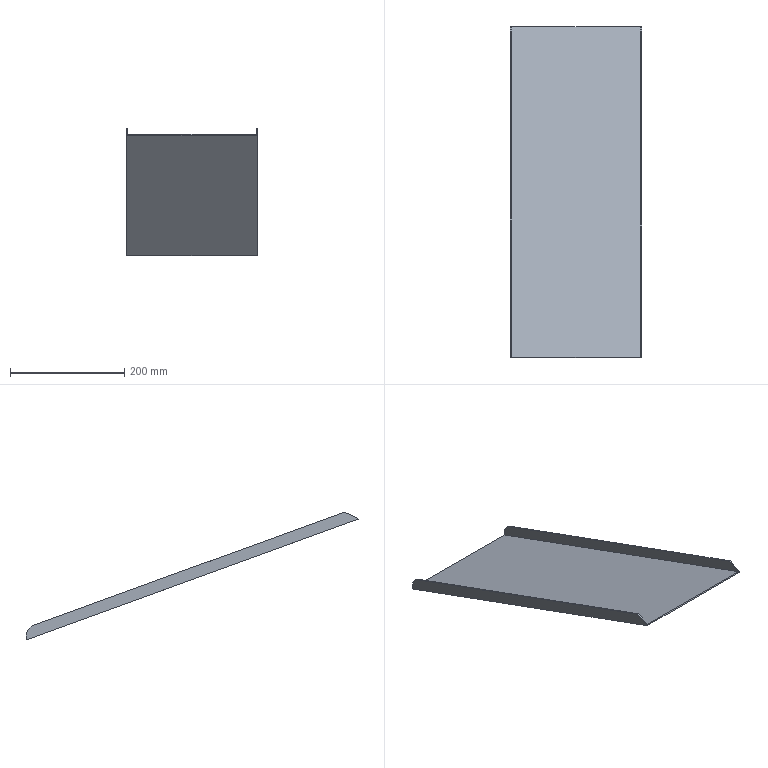Part | NX | features solid 2 | 1 solid | 15 faces | box 229.044 x 580.567 x 223.508 mm | volume 325645 mm3 | plane 13 | cylinder 2 | commonest cylinder face diameters 40 x2
STEP:
#1=CARTESIAN_POINT('',(-7.044,820.,-511.765));
#2=VERTEX_POINT('',#1);
#3=CARTESIAN_POINT('',(218.,820.,-511.765));
#4=VERTEX_POINT('',#3);
#5=CARTESIAN_POINT('',(-4.044,820.,-511.765));
#6=DIRECTION('',(-1.,0.,0.));
#7=VECTOR('',#6,1000.);
#8=LINE('',#5,#7);
#9=EDGE_CURVE('',#2,#4,#8,.F.);
#10=ORIENTED_EDGE('',*,*,#9,.F.);
#11=CARTESIAN_POINT('',(-7.044,820.,-509.637));
#12=VERTEX_POINT('',#11);
#13=CARTESIAN_POINT('',(-7.044,820.,-700.));
#14=DIRECTION('',(0.,0.,-1.));
#15=VECTOR('',#14,1000.);
#16=LINE('',#13,#15);
#17=EDGE_CURVE('',#2,#12,#16,.F.);
#18=ORIENTED_EDGE('',*,*,#17,.T.);
#19=CARTESIAN_POINT('',(218.,820.,-509.637));
#20=VERTEX_POINT('',#19);
#21=CARTESIAN_POINT('',(1065.,820.,-509.637));
#22=DIRECTION('',(1.,0.,0.));
#23=VECTOR('',#22,1000.);
#24=LINE('',#21,#23);
#25=EDGE_CURVE('',#20,#12,#24,.F.);
#26=ORIENTED_EDGE('',*,*,#25,.F.);
#27=CARTESIAN_POINT('',(218.,820.,-700.));
#28=DIRECTION('',(0.,0.,-1.));
#29=VECTOR('',#28,1000.);
#30=LINE('',#27,#29);
#31=EDGE_CURVE('',#4,#20,#30,.F.);
#32=ORIENTED_EDGE('',*,*,#31,.F.);
#33=EDGE_LOOP('',(#10,#18,#26,#32));
#34=FACE_BOUND('',#33,.T.);
#35=CARTESIAN_POINT('',(1065.,820.,-700.));
#36=DIRECTION('',(0.,-1.,0.));
#37=DIRECTION('',(-1.,0.,0.));
#38=AXIS2_PLACEMENT_3D('',#35,#36,#37);
#39=PLANE('',#38);
#40=ADVANCED_FACE('',(#34),#39,.F.);
#41=CARTESIAN_POINT('',(218.,241.366,-299.031));
#42=VERTEX_POINT('',#41);
#43=CARTESIAN_POINT('',(-7.044,241.366,-299.031));
#44=VERTEX_POINT('',#43);
#45=CARTESIAN_POINT('',(-4.044,241.366,-299.031));
#46=DIRECTION('',(-1.,0.,0.));
#47=VECTOR('',#46,1000.);
#48=LINE('',#45,#47);
#49=EDGE_CURVE('',#42,#44,#48,.T.);
#50=ORIENTED_EDGE('',*,*,#49,.T.);
#51=CARTESIAN_POINT('',(-7.044,240.682,-300.911));
#52=VERTEX_POINT('',#51);
#53=CARTESIAN_POINT('',(-7.044,240.682,-300.911));
#54=DIRECTION('',(0.,-0.342,-0.9397));
#55=VECTOR('',#54,1000.);
#56=LINE('',#53,#55);
#57=EDGE_CURVE('',#44,#52,#56,.T.);
#58=ORIENTED_EDGE('',*,*,#57,.T.);
#59=CARTESIAN_POINT('',(220.,240.682,-300.911));
#60=VERTEX_POINT('',#59);
#61=CARTESIAN_POINT('',(-4.044,240.682,-300.911));
#62=DIRECTION('',(-1.,0.,0.));
#63=VECTOR('',#62,1000.);
#64=LINE('',#61,#63);
#65=EDGE_CURVE('',#60,#52,#64,.T.);
#66=ORIENTED_EDGE('',*,*,#65,.F.);
#67=CARTESIAN_POINT('',(220.,241.366,-299.031));
#68=VERTEX_POINT('',#67);
#69=CARTESIAN_POINT('',(220.,241.366,-299.031));
#70=DIRECTION('',(0.,-0.342,-0.9397));
#71=VECTOR('',#70,1000.);
#72=LINE('',#69,#71);
#73=EDGE_CURVE('',#68,#60,#72,.T.);
#74=ORIENTED_EDGE('',*,*,#73,.F.);
#75=CARTESIAN_POINT('',(-4.044,241.366,-299.031));
#76=DIRECTION('',(-1.,0.,0.));
#77=VECTOR('',#76,1000.);
#78=LINE('',#75,#77);
#79=EDGE_CURVE('',#68,#42,#78,.T.);
#80=ORIENTED_EDGE('',*,*,#79,.T.);
#81=EDGE_LOOP('',(#50,#58,#66,#74,#80));
#82=FACE_BOUND('',#81,.T.);
#83=CARTESIAN_POINT('',(220.,240.682,-300.911));
#84=DIRECTION('',(0.,-0.9397,0.342));
#85=DIRECTION('',(0.,0.342,0.9397));
#86=AXIS2_PLACEMENT_3D('',#83,#84,#85);
#87=PLANE('',#86);
#88=ADVANCED_FACE('',(#82),#87,.T.);
#89=CARTESIAN_POINT('',(-7.044,1206.032,-650.141));
#90=DIRECTION('',(0.,0.9397,-0.342));
#91=VECTOR('',#90,1000.);
#92=LINE('',#89,#91);
#93=EDGE_CURVE('',#44,#12,#92,.T.);
#94=ORIENTED_EDGE('',*,*,#93,.F.);
#95=ORIENTED_EDGE('',*,*,#49,.F.);
#96=CARTESIAN_POINT('',(218.,1206.032,-650.141));
#97=DIRECTION('',(0.,0.9397,-0.342));
#98=VECTOR('',#97,1000.);
#99=LINE('',#96,#98);
#100=EDGE_CURVE('',#42,#20,#99,.T.);
#101=ORIENTED_EDGE('',*,*,#100,.T.);
#102=ORIENTED_EDGE('',*,*,#25,.T.);
#103=EDGE_LOOP('',(#94,#95,#101,#102));
#104=FACE_BOUND('',#103,.T.);
#105=CARTESIAN_POINT('',(-4.044,1206.032,-650.141));
#106=DIRECTION('',(0.,-0.342,-0.9397));
#107=DIRECTION('',(-1.,0.,0.));
#108=AXIS2_PLACEMENT_3D('',#105,#106,#107);
#109=PLANE('',#108);
#110=ADVANCED_FACE('',(#104),#109,.F.);
#111=CARTESIAN_POINT('',(220.,820.,-511.765));
#112=VERTEX_POINT('',#111);
#113=CARTESIAN_POINT('',(220.,1205.348,-652.02));
#114=DIRECTION('',(0.,-0.9397,0.342));
#115=VECTOR('',#114,1000.);
#116=LINE('',#113,#115);
#117=EDGE_CURVE('',#112,#60,#116,.T.);
#118=ORIENTED_EDGE('',*,*,#117,.F.);
#119=CARTESIAN_POINT('',(220.,808.047,-486.131));
#120=VERTEX_POINT('',#119);
#121=CARTESIAN_POINT('',(220.,801.206,-504.925));
#122=DIRECTION('',(-1.,0.,0.));
#123=DIRECTION('',(0.,0.,1.));
#124=AXIS2_PLACEMENT_3D('',#121,#122,#123);
#125=CIRCLE('',#124,20.);
#126=EDGE_CURVE('',#112,#120,#125,.F.);
#127=ORIENTED_EDGE('',*,*,#126,.T.);
#128=CARTESIAN_POINT('',(220.,264.437,-288.273));
#129=VERTEX_POINT('',#128);
#130=CARTESIAN_POINT('',(220.,826.84,-492.971));
#131=DIRECTION('',(0.,-0.9397,0.342));
#132=VECTOR('',#131,1000.);
#133=LINE('',#130,#132);
#134=EDGE_CURVE('',#120,#129,#133,.T.);
#135=ORIENTED_EDGE('',*,*,#134,.T.);
#136=CARTESIAN_POINT('',(220.,241.366,-299.031));
#137=DIRECTION('',(0.,-0.9063,-0.4226));
#138=VECTOR('',#137,1000.);
#139=LINE('',#136,#138);
#140=EDGE_CURVE('',#129,#68,#139,.T.);
#141=ORIENTED_EDGE('',*,*,#140,.T.);
#142=ORIENTED_EDGE('',*,*,#73,.T.);
#143=EDGE_LOOP('',(#118,#127,#135,#141,#142));
#144=FACE_BOUND('',#143,.T.);
#145=CARTESIAN_POINT('',(220.,1206.032,-650.141));
#146=DIRECTION('',(1.,0.,0.));
#147=DIRECTION('',(0.,0.,-1.));
#148=AXIS2_PLACEMENT_3D('',#145,#146,#147);
#149=PLANE('',#148);
#150=ADVANCED_FACE('',(#144),#149,.T.);
#151=CARTESIAN_POINT('',(-9.044,808.047,-486.131));
#152=VERTEX_POINT('',#151);
#153=CARTESIAN_POINT('',(-9.044,820.,-511.765));
#154=VERTEX_POINT('',#153);
#155=CARTESIAN_POINT('',(-9.044,801.206,-504.925));
#156=DIRECTION('',(-1.,0.,0.));
#157=DIRECTION('',(0.,0.,1.));
#158=AXIS2_PLACEMENT_3D('',#155,#156,#157);
#159=CIRCLE('',#158,20.);
#160=EDGE_CURVE('',#152,#154,#159,.T.);
#161=ORIENTED_EDGE('',*,*,#160,.T.);
#162=CARTESIAN_POINT('',(-9.044,240.639,-300.895));
#163=VERTEX_POINT('',#162);
#164=CARTESIAN_POINT('',(-9.044,1205.348,-652.02));
#165=DIRECTION('',(0.,-0.9397,0.342));
#166=VECTOR('',#165,1000.);
#167=LINE('',#164,#166);
#168=EDGE_CURVE('',#154,#163,#167,.T.);
#169=ORIENTED_EDGE('',*,*,#168,.T.);
#170=CARTESIAN_POINT('',(-9.044,241.323,-299.015));
#171=VERTEX_POINT('',#170);
#172=CARTESIAN_POINT('',(-9.044,240.639,-300.895));
#173=DIRECTION('',(0.,0.342,0.9397));
#174=VECTOR('',#173,1000.);
#175=LINE('',#172,#174);
#176=EDGE_CURVE('',#163,#171,#175,.T.);
#177=ORIENTED_EDGE('',*,*,#176,.T.);
#178=CARTESIAN_POINT('',(-9.044,264.394,-288.257));
#179=VERTEX_POINT('',#178);
#180=CARTESIAN_POINT('',(-9.044,635.157,-115.368));
#181=DIRECTION('',(0.,0.9063,0.4226));
#182=VECTOR('',#181,1000.);
#183=LINE('',#180,#182);
#184=EDGE_CURVE('',#171,#179,#183,.T.);
#185=ORIENTED_EDGE('',*,*,#184,.T.);
#186=CARTESIAN_POINT('',(-9.044,826.84,-492.971));
#187=DIRECTION('',(0.,-0.9397,0.342));
#188=VECTOR('',#187,1000.);
#189=LINE('',#186,#188);
#190=EDGE_CURVE('',#152,#179,#189,.T.);
#191=ORIENTED_EDGE('',*,*,#190,.F.);
#192=EDGE_LOOP('',(#161,#169,#177,#185,#191));
#193=FACE_BOUND('',#192,.T.);
#194=CARTESIAN_POINT('',(-9.044,1206.032,-650.141));
#195=DIRECTION('',(1.,0.,0.));
#196=DIRECTION('',(0.,0.,-1.));
#197=AXIS2_PLACEMENT_3D('',#194,#195,#196);
#198=PLANE('',#197);
#199=ADVANCED_FACE('',(#193),#198,.F.);
#200=CARTESIAN_POINT('',(-4.044,820.,-511.765));
#201=DIRECTION('',(-1.,0.,0.));
#202=VECTOR('',#201,1000.);
#203=LINE('',#200,#202);
#204=EDGE_CURVE('',#154,#2,#203,.F.);
#205=ORIENTED_EDGE('',*,*,#204,.T.);
#206=ORIENTED_EDGE('',*,*,#9,.T.);
#207=CARTESIAN_POINT('',(220.,820.,-511.765));
#208=DIRECTION('',(1.,0.,0.));
#209=VECTOR('',#208,1000.);
#210=LINE('',#207,#209);
#211=EDGE_CURVE('',#112,#4,#210,.F.);
#212=ORIENTED_EDGE('',*,*,#211,.F.);
#213=ORIENTED_EDGE('',*,*,#117,.T.);
#214=ORIENTED_EDGE('',*,*,#65,.T.);
#215=CARTESIAN_POINT('',(-7.044,240.639,-300.895));
#216=VERTEX_POINT('',#215);
#217=CARTESIAN_POINT('',(-7.044,820.,-511.765));
#218=DIRECTION('',(0.,-0.9397,0.342));
#219=VECTOR('',#218,1000.);
#220=LINE('',#217,#219);
#221=EDGE_CURVE('',#52,#216,#220,.T.);
#222=ORIENTED_EDGE('',*,*,#221,.T.);
#223=CARTESIAN_POINT('',(-9.044,240.639,-300.895));
#224=DIRECTION('',(1.,0.,0.));
#225=VECTOR('',#224,1000.);
#226=LINE('',#223,#225);
#227=EDGE_CURVE('',#163,#216,#226,.T.);
#228=ORIENTED_EDGE('',*,*,#227,.F.);
#229=ORIENTED_EDGE('',*,*,#168,.F.);
#230=EDGE_LOOP('',(#205,#206,#212,#213,#214,#222,#228,#229));
#231=FACE_BOUND('',#230,.T.);
#232=CARTESIAN_POINT('',(-4.044,1205.348,-652.02));
#233=DIRECTION('',(0.,-0.342,-0.9397));
#234=DIRECTION('',(-1.,0.,0.));
#235=AXIS2_PLACEMENT_3D('',#232,#233,#234);
#236=PLANE('',#235);
#237=ADVANCED_FACE('',(#231),#236,.T.);
#238=CARTESIAN_POINT('',(218.,808.047,-486.131));
#239=VERTEX_POINT('',#238);
#240=CARTESIAN_POINT('',(218.,264.437,-288.273));
#241=VERTEX_POINT('',#240);
#242=CARTESIAN_POINT('',(218.,826.84,-492.971));
#243=DIRECTION('',(0.,-0.9397,0.342));
#244=VECTOR('',#243,1000.);
#245=LINE('',#242,#244);
#246=EDGE_CURVE('',#239,#241,#245,.T.);
#247=ORIENTED_EDGE('',*,*,#246,.T.);
#248=CARTESIAN_POINT('',(220.,264.437,-288.273));
#249=DIRECTION('',(1.,0.,0.));
#250=VECTOR('',#249,1000.);
#251=LINE('',#248,#250);
#252=EDGE_CURVE('',#241,#129,#251,.T.);
#253=ORIENTED_EDGE('',*,*,#252,.T.);
#254=ORIENTED_EDGE('',*,*,#134,.F.);
#255=CARTESIAN_POINT('',(220.,808.047,-486.131));
#256=DIRECTION('',(-1.,0.,0.));
#257=VECTOR('',#256,1000.);
#258=LINE('',#255,#257);
#259=EDGE_CURVE('',#120,#239,#258,.T.);
#260=ORIENTED_EDGE('',*,*,#259,.T.);
#261=EDGE_LOOP('',(#247,#253,#254,#260));
#262=FACE_BOUND('',#261,.T.);
#263=CARTESIAN_POINT('',(220.,826.84,-492.971));
#264=DIRECTION('',(0.,-0.342,-0.9397));
#265=DIRECTION('',(0.,-0.9397,0.342));
#266=AXIS2_PLACEMENT_3D('',#263,#264,#265);
#267=PLANE('',#266);
#268=ADVANCED_FACE('',(#262),#267,.F.);
#269=CARTESIAN_POINT('',(218.,801.206,-504.925));
#270=DIRECTION('',(-1.,0.,0.));
#271=DIRECTION('',(0.,0.,1.));
#272=AXIS2_PLACEMENT_3D('',#269,#270,#271);
#273=CIRCLE('',#272,20.);
#274=EDGE_CURVE('',#239,#4,#273,.T.);
#275=ORIENTED_EDGE('',*,*,#274,.T.);
#276=ORIENTED_EDGE('',*,*,#31,.T.);
#277=ORIENTED_EDGE('',*,*,#100,.F.);
#278=CARTESIAN_POINT('',(218.,635.171,-115.397));
#279=DIRECTION('',(0.,0.9063,0.4226));
#280=VECTOR('',#279,1000.);
#281=LINE('',#278,#280);
#282=EDGE_CURVE('',#42,#241,#281,.T.);
#283=ORIENTED_EDGE('',*,*,#282,.T.);
#284=ORIENTED_EDGE('',*,*,#246,.F.);
#285=EDGE_LOOP('',(#275,#276,#277,#283,#284));
#286=FACE_BOUND('',#285,.T.);
#287=CARTESIAN_POINT('',(218.,820.,-511.765));
#288=DIRECTION('',(-1.,0.,0.));
#289=DIRECTION('',(0.,0.,1.));
#290=AXIS2_PLACEMENT_3D('',#287,#288,#289);
#291=PLANE('',#290);
#292=ADVANCED_FACE('',(#286),#291,.T.);
#293=ORIENTED_EDGE('',*,*,#126,.F.);
#294=ORIENTED_EDGE('',*,*,#211,.T.);
#295=ORIENTED_EDGE('',*,*,#274,.F.);
#296=ORIENTED_EDGE('',*,*,#259,.F.);
#297=EDGE_LOOP('',(#293,#294,#295,#296));
#298=FACE_BOUND('',#297,.T.);
#299=CARTESIAN_POINT('',(220.,801.206,-504.925));
#300=DIRECTION('',(-1.,0.,0.));
#301=DIRECTION('',(0.,0.,1.));
#302=AXIS2_PLACEMENT_3D('',#299,#300,#301);
#303=CYLINDRICAL_SURFACE('',#302,20.);
#304=ADVANCED_FACE('',(#298),#303,.T.);
#305=ORIENTED_EDGE('',*,*,#140,.F.);
#306=ORIENTED_EDGE('',*,*,#252,.F.);
#307=ORIENTED_EDGE('',*,*,#282,.F.);
#308=ORIENTED_EDGE('',*,*,#79,.F.);
#309=EDGE_LOOP('',(#305,#306,#307,#308));
#310=FACE_BOUND('',#309,.T.);
#311=CARTESIAN_POINT('',(220.,241.366,-299.031));
#312=DIRECTION('',(0.,-0.4226,0.9063));
#313=DIRECTION('',(0.,-0.9063,-0.4226));
#314=AXIS2_PLACEMENT_3D('',#311,#312,#313);
#315=PLANE('',#314);
#316=ADVANCED_FACE('',(#310),#315,.T.);
#317=ORIENTED_EDGE('',*,*,#190,.T.);
#318=CARTESIAN_POINT('',(-7.044,264.394,-288.257));
#319=VERTEX_POINT('',#318);
#320=CARTESIAN_POINT('',(-9.044,264.394,-288.257));
#321=DIRECTION('',(-1.,0.,0.));
#322=VECTOR('',#321,1000.);
#323=LINE('',#320,#322);
#324=EDGE_CURVE('',#179,#319,#323,.F.);
#325=ORIENTED_EDGE('',*,*,#324,.T.);
#326=CARTESIAN_POINT('',(-7.044,808.047,-486.131));
#327=VERTEX_POINT('',#326);
#328=CARTESIAN_POINT('',(-7.044,826.84,-492.971));
#329=DIRECTION('',(0.,-0.9397,0.342));
#330=VECTOR('',#329,1000.);
#331=LINE('',#328,#330);
#332=EDGE_CURVE('',#327,#319,#331,.T.);
#333=ORIENTED_EDGE('',*,*,#332,.F.);
#334=CARTESIAN_POINT('',(-9.044,808.047,-486.131));
#335=DIRECTION('',(-1.,0.,0.));
#336=VECTOR('',#335,1000.);
#337=LINE('',#334,#336);
#338=EDGE_CURVE('',#327,#152,#337,.T.);
#339=ORIENTED_EDGE('',*,*,#338,.T.);
#340=EDGE_LOOP('',(#317,#325,#333,#339));
#341=FACE_BOUND('',#340,.T.);
#342=CARTESIAN_POINT('',(-9.044,826.84,-492.971));
#343=DIRECTION('',(0.,-0.342,-0.9397));
#344=DIRECTION('',(0.,-0.9397,0.342));
#345=AXIS2_PLACEMENT_3D('',#342,#343,#344);
#346=PLANE('',#345);
#347=ADVANCED_FACE('',(#341),#346,.F.);
#348=ORIENTED_EDGE('',*,*,#17,.F.);
#349=CARTESIAN_POINT('',(-7.044,801.206,-504.925));
#350=DIRECTION('',(-1.,0.,0.));
#351=DIRECTION('',(0.,0.,1.));
#352=AXIS2_PLACEMENT_3D('',#349,#350,#351);
#353=CIRCLE('',#352,20.);
#354=EDGE_CURVE('',#2,#327,#353,.F.);
#355=ORIENTED_EDGE('',*,*,#354,.T.);
#356=ORIENTED_EDGE('',*,*,#332,.T.);
#357=CARTESIAN_POINT('',(-7.044,241.323,-299.015));
#358=VERTEX_POINT('',#357);
#359=CARTESIAN_POINT('',(-7.044,264.394,-288.257));
#360=DIRECTION('',(0.,-0.9063,-0.4226));
#361=VECTOR('',#360,1000.);
#362=LINE('',#359,#361);
#363=EDGE_CURVE('',#319,#358,#362,.T.);
#364=ORIENTED_EDGE('',*,*,#363,.T.);
#365=CARTESIAN_POINT('',(-7.044,240.639,-300.895));
#366=DIRECTION('',(0.,0.342,0.9397));
#367=VECTOR('',#366,1000.);
#368=LINE('',#365,#367);
#369=EDGE_CURVE('',#216,#358,#368,.T.);
#370=ORIENTED_EDGE('',*,*,#369,.F.);
#371=ORIENTED_EDGE('',*,*,#221,.F.);
#372=ORIENTED_EDGE('',*,*,#57,.F.);
#373=ORIENTED_EDGE('',*,*,#93,.T.);
#374=EDGE_LOOP('',(#348,#355,#356,#364,#370,#371,#372,#373));
#375=FACE_BOUND('',#374,.T.);
#376=CARTESIAN_POINT('',(-7.044,820.,-511.765));
#377=DIRECTION('',(-1.,0.,0.));
#378=DIRECTION('',(0.,0.,1.));
#379=AXIS2_PLACEMENT_3D('',#376,#377,#378);
#380=PLANE('',#379);
#381=ADVANCED_FACE('',(#375),#380,.F.);
#382=ORIENTED_EDGE('',*,*,#369,.T.);
#383=CARTESIAN_POINT('',(-9.044,241.323,-299.015));
#384=DIRECTION('',(-1.,0.,0.));
#385=VECTOR('',#384,1000.);
#386=LINE('',#383,#385);
#387=EDGE_CURVE('',#358,#171,#386,.T.);
#388=ORIENTED_EDGE('',*,*,#387,.T.);
#389=ORIENTED_EDGE('',*,*,#176,.F.);
#390=ORIENTED_EDGE('',*,*,#227,.T.);
#391=EDGE_LOOP('',(#382,#388,#389,#390));
#392=FACE_BOUND('',#391,.T.);
#393=CARTESIAN_POINT('',(-9.044,240.639,-300.895));
#394=DIRECTION('',(0.,-0.9397,0.342));
#395=DIRECTION('',(0.,0.342,0.9397));
#396=AXIS2_PLACEMENT_3D('',#393,#394,#395);
#397=PLANE('',#396);
#398=ADVANCED_FACE('',(#392),#397,.T.);
#399=ORIENTED_EDGE('',*,*,#160,.F.);
#400=ORIENTED_EDGE('',*,*,#338,.F.);
#401=ORIENTED_EDGE('',*,*,#354,.F.);
#402=ORIENTED_EDGE('',*,*,#204,.F.);
#403=EDGE_LOOP('',(#399,#400,#401,#402));
#404=FACE_BOUND('',#403,.T.);
#405=CARTESIAN_POINT('',(-9.044,801.206,-504.925));
#406=DIRECTION('',(1.,0.,0.));
#407=DIRECTION('',(0.,0.,-1.));
#408=AXIS2_PLACEMENT_3D('',#405,#406,#407);
#409=CYLINDRICAL_SURFACE('',#408,20.);
#410=ADVANCED_FACE('',(#404),#409,.T.);
#411=ORIENTED_EDGE('',*,*,#184,.F.);
#412=ORIENTED_EDGE('',*,*,#387,.F.);
#413=ORIENTED_EDGE('',*,*,#363,.F.);
#414=ORIENTED_EDGE('',*,*,#324,.F.);
#415=EDGE_LOOP('',(#411,#412,#413,#414));
#416=FACE_BOUND('',#415,.T.);
#417=CARTESIAN_POINT('',(-9.044,264.394,-288.257));
#418=DIRECTION('',(0.,-0.4226,0.9063));
#419=DIRECTION('',(0.,-0.9063,-0.4226));
#420=AXIS2_PLACEMENT_3D('',#417,#418,#419);
#421=PLANE('',#420);
#422=ADVANCED_FACE('',(#416),#421,.T.);
#423=CLOSED_SHELL('',(#40,#88,#110,#150,#199,#237,#268,#292,#304,#316,#347,#381,#398,#410,#422));
#424=MANIFOLD_SOLID_BREP('',#423);
#425=(LENGTH_UNIT()NAMED_UNIT(*)SI_UNIT(.MILLI.,.METRE.));
#426=UNCERTAINTY_MEASURE_WITH_UNIT(LENGTH_MEASURE(0.00001),#425,'','');
#427=(NAMED_UNIT(*)PLANE_ANGLE_UNIT()SI_UNIT($,.RADIAN.));
#428=(NAMED_UNIT(*)SI_UNIT($,.STERADIAN.)SOLID_ANGLE_UNIT());
#429=(GEOMETRIC_REPRESENTATION_CONTEXT(3)GLOBAL_UNCERTAINTY_ASSIGNED_CONTEXT((#426))GLOBAL_UNIT_ASSIGNED_CONTEXT((#425,#427,#428))REPRESENTATION_CONTEXT('',''));
#430=ADVANCED_BREP_SHAPE_REPRESENTATION('',(#424),#429);